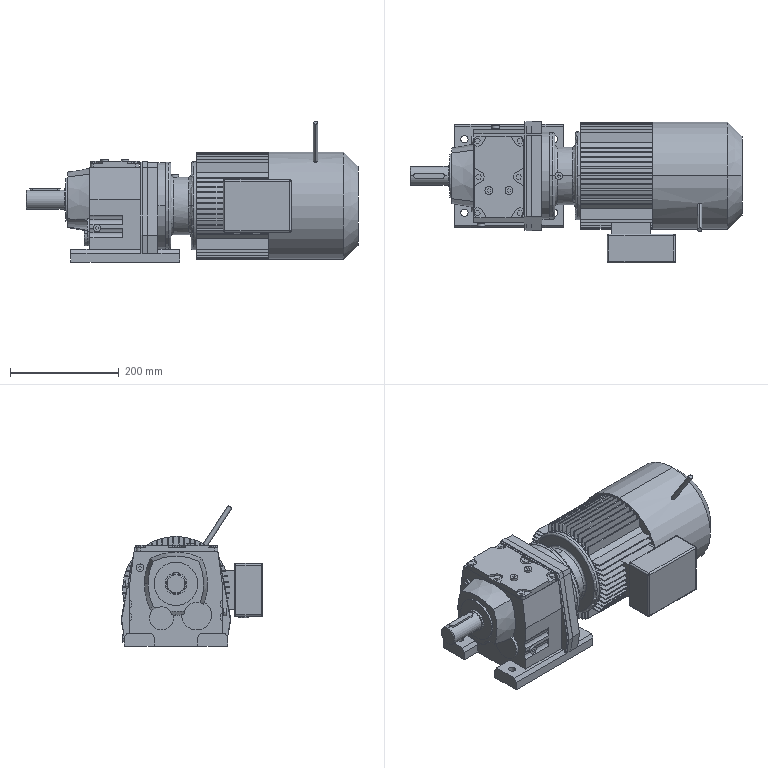Part | STEP file | R57DRE80M4_BE-M1-0-0.75KW | 16 solids | 650 faces | box 610.5 x 261 x 258.648 mm | volume 14119435 mm3 | plane 504 | cylinder 107 | sphere 20 | cone 11 | torus 8 | commonest cylinder face diameters 14 x14 6 x12 8 x12 9 x8 13.5 x8 20 x7